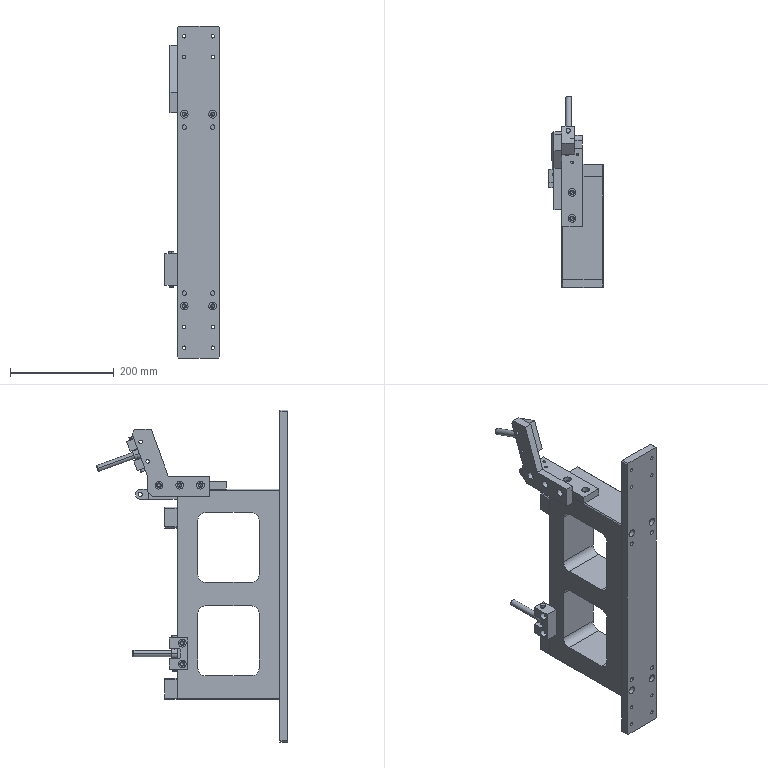Part | SolidWorks | 13 solids | 392 faces | box 105 x 368.457 x 640 mm | volume 5118898 mm3 | cylinder 214 | plane 138 | cone 40 | commonest cylinder face diameters 6.8 x38 15 x38 9 x30 6.6 x16 11 x16 8 x12